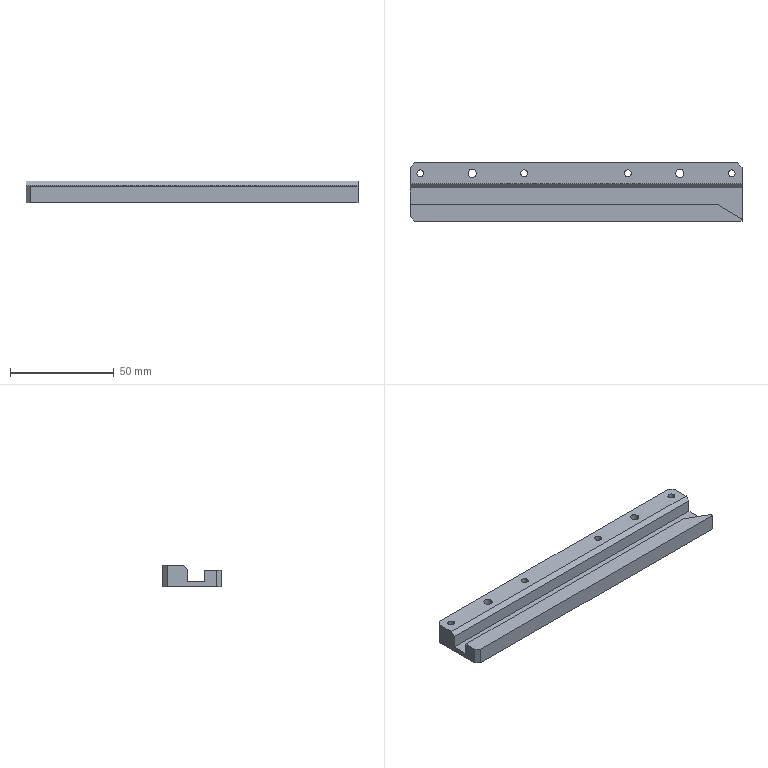Part | STEP file | QA-AD09 | 1 solid | 29 faces | box 160 x 28 x 10.5 mm | volume 32238 mm3 | plane 15 | cylinder 14 | commonest cylinder face diameters 3.3 x8 4 x5 2 x1